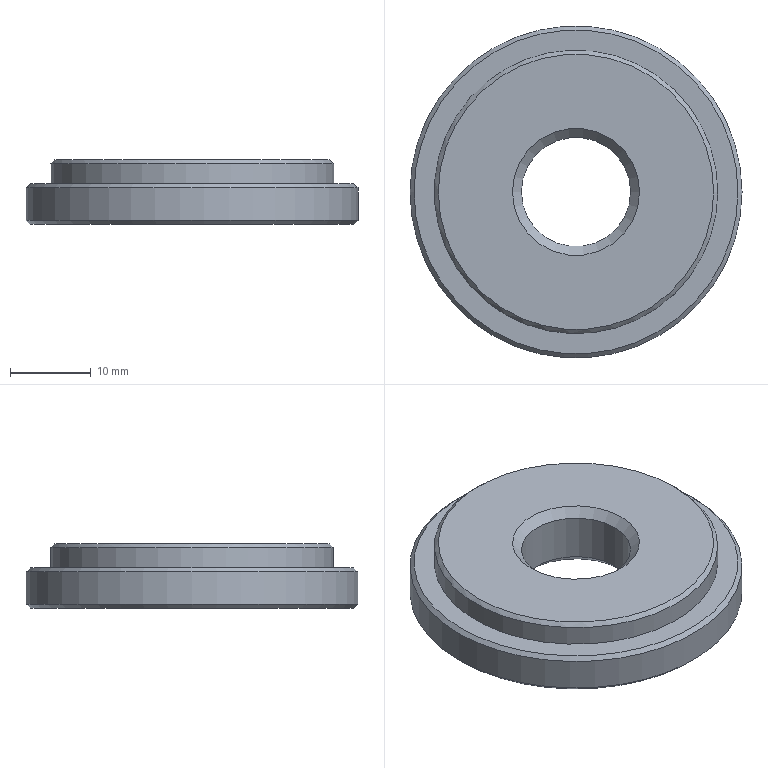Part | NX | features CYLINDER 2, CHAMFER 1, DATUM_CSYS 1, HOLE PACKAGE 1, SIMPLE HOLE 1 | 1 solid | 11 faces | box 41 x 41 x 8 mm | volume 8243 mm3 | cone 5 | plane 3 | cylinder 3 | commonest cylinder face diameters 13.5 x1 35 x1 41 x1
STEP:
#1=CARTESIAN_POINT('',(20.,0.,5.));
#2=VERTEX_POINT('',#1);
#3=CARTESIAN_POINT('',(0.,0.,5.));
#4=DIRECTION('',(0.,0.,1.));
#5=DIRECTION('',(1.,0.,0.));
#6=AXIS2_PLACEMENT_3D('',#3,#4,#5);
#7=CIRCLE('',#6,20.);
#8=EDGE_CURVE('',#2,#2,#7,.T.);
#9=ORIENTED_EDGE('',*,*,#8,.T.);
#10=EDGE_LOOP('',(#9));
#11=FACE_BOUND('',#10,.T.);
#12=CARTESIAN_POINT('',(17.5,0.,5.));
#13=VERTEX_POINT('',#12);
#14=CARTESIAN_POINT('',(0.,0.,5.));
#15=DIRECTION('',(0.,0.,1.));
#16=DIRECTION('',(1.,0.,0.));
#17=AXIS2_PLACEMENT_3D('',#14,#15,#16);
#18=CIRCLE('',#17,17.5);
#19=EDGE_CURVE('',#13,#13,#18,.T.);
#20=ORIENTED_EDGE('',*,*,#19,.F.);
#21=EDGE_LOOP('',(#20));
#22=FACE_BOUND('',#21,.T.);
#23=CARTESIAN_POINT('',(0.,0.,5.));
#24=DIRECTION('',(0.,0.,1.));
#25=DIRECTION('',(1.,0.,0.));
#26=AXIS2_PLACEMENT_3D('',#23,#24,#25);
#27=PLANE('',#26);
#28=ADVANCED_FACE('',(#11,#22),#27,.T.);
#29=CARTESIAN_POINT('',(-7.85,0.,0.));
#30=VERTEX_POINT('',#29);
#31=CARTESIAN_POINT('',(0.,0.,0.));
#32=DIRECTION('',(0.,0.,-1.));
#33=DIRECTION('',(-1.,0.,0.));
#34=AXIS2_PLACEMENT_3D('',#31,#32,#33);
#35=CIRCLE('',#34,7.85);
#36=EDGE_CURVE('',#30,#30,#35,.F.);
#37=ORIENTED_EDGE('',*,*,#36,.T.);
#38=EDGE_LOOP('',(#37));
#39=FACE_BOUND('',#38,.T.);
#40=CARTESIAN_POINT('',(-20.,0.,0.));
#41=VERTEX_POINT('',#40);
#42=CARTESIAN_POINT('',(0.,0.,0.));
#43=DIRECTION('',(0.,0.,-1.));
#44=DIRECTION('',(-1.,0.,0.));
#45=AXIS2_PLACEMENT_3D('',#42,#43,#44);
#46=CIRCLE('',#45,20.);
#47=EDGE_CURVE('',#41,#41,#46,.T.);
#48=ORIENTED_EDGE('',*,*,#47,.T.);
#49=EDGE_LOOP('',(#48));
#50=FACE_BOUND('',#49,.T.);
#51=CARTESIAN_POINT('',(0.,0.,0.));
#52=DIRECTION('',(0.,0.,-1.));
#53=DIRECTION('',(-1.,0.,0.));
#54=AXIS2_PLACEMENT_3D('',#51,#52,#53);
#55=PLANE('',#54);
#56=ADVANCED_FACE('',(#39,#50),#55,.T.);
#57=CARTESIAN_POINT('',(20.5,0.,4.5));
#58=VERTEX_POINT('',#57);
#59=CARTESIAN_POINT('',(0.,0.,4.5));
#60=DIRECTION('',(0.,0.,1.));
#61=DIRECTION('',(1.,0.,0.));
#62=AXIS2_PLACEMENT_3D('',#59,#60,#61);
#63=CIRCLE('',#62,20.5);
#64=EDGE_CURVE('',#58,#58,#63,.F.);
#65=ORIENTED_EDGE('',*,*,#64,.T.);
#66=EDGE_LOOP('',(#65));
#67=FACE_BOUND('',#66,.T.);
#68=CARTESIAN_POINT('',(-20.5,0.,0.5));
#69=VERTEX_POINT('',#68);
#70=CARTESIAN_POINT('',(0.,0.,0.5));
#71=DIRECTION('',(0.,0.,-1.));
#72=DIRECTION('',(-1.,0.,0.));
#73=AXIS2_PLACEMENT_3D('',#70,#71,#72);
#74=CIRCLE('',#73,20.5);
#75=EDGE_CURVE('',#69,#69,#74,.F.);
#76=ORIENTED_EDGE('',*,*,#75,.T.);
#77=EDGE_LOOP('',(#76));
#78=FACE_BOUND('',#77,.T.);
#79=CARTESIAN_POINT('',(0.,0.,0.));
#80=DIRECTION('',(0.,0.,1.));
#81=DIRECTION('',(1.,0.,0.));
#82=AXIS2_PLACEMENT_3D('',#79,#80,#81);
#83=CYLINDRICAL_SURFACE('',#82,20.5);
#84=ADVANCED_FACE('',(#67,#78),#83,.T.);
#85=CARTESIAN_POINT('',(7.85,0.,8.));
#86=VERTEX_POINT('',#85);
#87=CARTESIAN_POINT('',(0.,0.,8.));
#88=DIRECTION('',(0.,0.,1.));
#89=DIRECTION('',(1.,0.,0.));
#90=AXIS2_PLACEMENT_3D('',#87,#88,#89);
#91=CIRCLE('',#90,7.85);
#92=EDGE_CURVE('',#86,#86,#91,.F.);
#93=ORIENTED_EDGE('',*,*,#92,.T.);
#94=EDGE_LOOP('',(#93));
#95=FACE_BOUND('',#94,.T.);
#96=CARTESIAN_POINT('',(17.,0.,8.));
#97=VERTEX_POINT('',#96);
#98=CARTESIAN_POINT('',(0.,0.,8.));
#99=DIRECTION('',(0.,0.,1.));
#100=DIRECTION('',(1.,0.,0.));
#101=AXIS2_PLACEMENT_3D('',#98,#99,#100);
#102=CIRCLE('',#101,17.);
#103=EDGE_CURVE('',#97,#97,#102,.T.);
#104=ORIENTED_EDGE('',*,*,#103,.T.);
#105=EDGE_LOOP('',(#104));
#106=FACE_BOUND('',#105,.T.);
#107=CARTESIAN_POINT('',(0.,0.,8.));
#108=DIRECTION('',(0.,0.,1.));
#109=DIRECTION('',(1.,0.,0.));
#110=AXIS2_PLACEMENT_3D('',#107,#108,#109);
#111=PLANE('',#110);
#112=ADVANCED_FACE('',(#95,#106),#111,.T.);
#113=CARTESIAN_POINT('',(17.5,0.,7.5));
#114=VERTEX_POINT('',#113);
#115=CARTESIAN_POINT('',(0.,0.,7.5));
#116=DIRECTION('',(0.,0.,1.));
#117=DIRECTION('',(1.,0.,0.));
#118=AXIS2_PLACEMENT_3D('',#115,#116,#117);
#119=CIRCLE('',#118,17.5);
#120=EDGE_CURVE('',#114,#114,#119,.F.);
#121=ORIENTED_EDGE('',*,*,#120,.T.);
#122=EDGE_LOOP('',(#121));
#123=FACE_BOUND('',#122,.T.);
#124=ORIENTED_EDGE('',*,*,#19,.T.);
#125=EDGE_LOOP('',(#124));
#126=FACE_BOUND('',#125,.T.);
#127=CARTESIAN_POINT('',(0.,0.,5.));
#128=DIRECTION('',(0.,0.,1.));
#129=DIRECTION('',(1.,0.,0.));
#130=AXIS2_PLACEMENT_3D('',#127,#128,#129);
#131=CYLINDRICAL_SURFACE('',#130,17.5);
#132=ADVANCED_FACE('',(#123,#126),#131,.T.);
#133=ORIENTED_EDGE('',*,*,#103,.F.);
#134=EDGE_LOOP('',(#133));
#135=FACE_BOUND('',#134,.T.);
#136=ORIENTED_EDGE('',*,*,#120,.F.);
#137=EDGE_LOOP('',(#136));
#138=FACE_BOUND('',#137,.T.);
#139=CARTESIAN_POINT('',(0.,0.,7.5));
#140=DIRECTION('',(0.,0.,-1.));
#141=DIRECTION('',(-1.,0.,0.));
#142=AXIS2_PLACEMENT_3D('',#139,#140,#141);
#143=CONICAL_SURFACE('',#142,17.5,0.7854);
#144=ADVANCED_FACE('',(#135,#138),#143,.T.);
#145=ORIENTED_EDGE('',*,*,#8,.F.);
#146=EDGE_LOOP('',(#145));
#147=FACE_BOUND('',#146,.T.);
#148=ORIENTED_EDGE('',*,*,#64,.F.);
#149=EDGE_LOOP('',(#148));
#150=FACE_BOUND('',#149,.T.);
#151=CARTESIAN_POINT('',(0.,0.,4.5));
#152=DIRECTION('',(0.,0.,-1.));
#153=DIRECTION('',(-1.,0.,0.));
#154=AXIS2_PLACEMENT_3D('',#151,#152,#153);
#155=CONICAL_SURFACE('',#154,20.5,0.7854);
#156=ADVANCED_FACE('',(#147,#150),#155,.T.);
#157=ORIENTED_EDGE('',*,*,#47,.F.);
#158=EDGE_LOOP('',(#157));
#159=FACE_BOUND('',#158,.T.);
#160=ORIENTED_EDGE('',*,*,#75,.F.);
#161=EDGE_LOOP('',(#160));
#162=FACE_BOUND('',#161,.T.);
#163=CARTESIAN_POINT('',(0.,0.,0.5));
#164=DIRECTION('',(0.,0.,1.));
#165=DIRECTION('',(1.,0.,0.));
#166=AXIS2_PLACEMENT_3D('',#163,#164,#165);
#167=CONICAL_SURFACE('',#166,20.5,0.7854);
#168=ADVANCED_FACE('',(#159,#162),#167,.T.);
#169=CARTESIAN_POINT('',(6.75,0.,6.9));
#170=VERTEX_POINT('',#169);
#171=CARTESIAN_POINT('',(0.,0.,6.9));
#172=DIRECTION('',(0.,0.,1.));
#173=DIRECTION('',(1.,0.,0.));
#174=AXIS2_PLACEMENT_3D('',#171,#172,#173);
#175=CIRCLE('',#174,6.75);
#176=EDGE_CURVE('',#170,#170,#175,.T.);
#177=ORIENTED_EDGE('',*,*,#176,.T.);
#178=EDGE_LOOP('',(#177));
#179=FACE_BOUND('',#178,.T.);
#180=CARTESIAN_POINT('',(-6.75,0.,1.1));
#181=VERTEX_POINT('',#180);
#182=CARTESIAN_POINT('',(0.,0.,1.1));
#183=DIRECTION('',(0.,0.,-1.));
#184=DIRECTION('',(-1.,0.,0.));
#185=AXIS2_PLACEMENT_3D('',#182,#183,#184);
#186=CIRCLE('',#185,6.75);
#187=EDGE_CURVE('',#181,#181,#186,.T.);
#188=ORIENTED_EDGE('',*,*,#187,.T.);
#189=EDGE_LOOP('',(#188));
#190=FACE_BOUND('',#189,.T.);
#191=CARTESIAN_POINT('',(0.,0.,0.));
#192=DIRECTION('',(0.,0.,1.));
#193=DIRECTION('',(1.,0.,0.));
#194=AXIS2_PLACEMENT_3D('',#191,#192,#193);
#195=CYLINDRICAL_SURFACE('',#194,6.75);
#196=ADVANCED_FACE('',(#179,#190),#195,.F.);
#197=ORIENTED_EDGE('',*,*,#187,.F.);
#198=EDGE_LOOP('',(#197));
#199=FACE_BOUND('',#198,.T.);
#200=ORIENTED_EDGE('',*,*,#36,.F.);
#201=EDGE_LOOP('',(#200));
#202=FACE_BOUND('',#201,.T.);
#203=CARTESIAN_POINT('',(0.,0.,0.));
#204=DIRECTION('',(0.,0.,-1.));
#205=DIRECTION('',(-1.,0.,0.));
#206=AXIS2_PLACEMENT_3D('',#203,#204,#205);
#207=CONICAL_SURFACE('',#206,7.85,0.7854);
#208=ADVANCED_FACE('',(#199,#202),#207,.F.);
#209=ORIENTED_EDGE('',*,*,#92,.F.);
#210=EDGE_LOOP('',(#209));
#211=FACE_BOUND('',#210,.T.);
#212=ORIENTED_EDGE('',*,*,#176,.F.);
#213=EDGE_LOOP('',(#212));
#214=FACE_BOUND('',#213,.T.);
#215=CARTESIAN_POINT('',(0.,0.,6.9));
#216=DIRECTION('',(0.,0.,1.));
#217=DIRECTION('',(1.,0.,0.));
#218=AXIS2_PLACEMENT_3D('',#215,#216,#217);
#219=CONICAL_SURFACE('',#218,6.75,0.7854);
#220=ADVANCED_FACE('',(#211,#214),#219,.F.);
#221=CLOSED_SHELL('',(#28,#56,#84,#112,#132,#144,#156,#168,#196,#208,#220));
#222=MANIFOLD_SOLID_BREP('',#221);
#223=(LENGTH_UNIT()NAMED_UNIT(*)SI_UNIT(.MILLI.,.METRE.));
#224=UNCERTAINTY_MEASURE_WITH_UNIT(LENGTH_MEASURE(0.00001),#223,'','');
#225=(NAMED_UNIT(*)PLANE_ANGLE_UNIT()SI_UNIT($,.RADIAN.));
#226=(NAMED_UNIT(*)SI_UNIT($,.STERADIAN.)SOLID_ANGLE_UNIT());
#227=(GEOMETRIC_REPRESENTATION_CONTEXT(3)GLOBAL_UNCERTAINTY_ASSIGNED_CONTEXT((#224))GLOBAL_UNIT_ASSIGNED_CONTEXT((#223,#225,#226))REPRESENTATION_CONTEXT('',''));
#228=ADVANCED_BREP_SHAPE_REPRESENTATION('',(#222),#227);